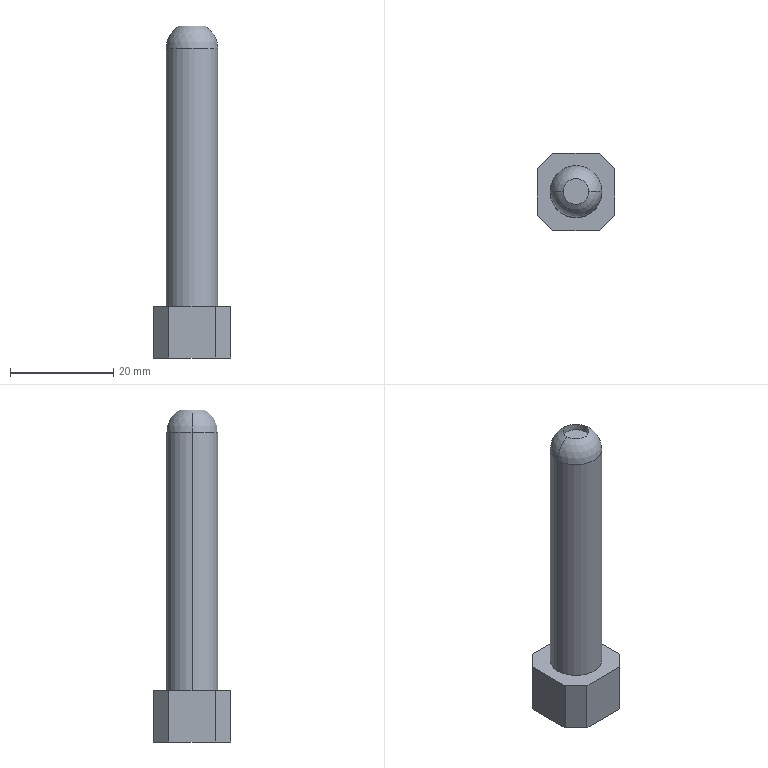Part | STEP file | Chamfer 1-56 | 1 solid | 17 faces | box 15 x 15 x 64.33 mm | volume 6226 mm3 | plane 11 | cylinder 4 | sphere 2 | commonest cylinder face diameters 5 x2 10 x2
STEP:
#1=CARTESIAN_POINT('',(-1533.738,1565.764,2844.751));
#2=VERTEX_POINT('',#1);
#3=CARTESIAN_POINT('',(-1528.738,1565.764,2844.751));
#4=VERTEX_POINT('',#3);
#5=CARTESIAN_POINT('',(-1531.238,1565.764,2844.751));
#6=DIRECTION('',(0.,0.,1.));
#7=DIRECTION('',(1.,0.,0.));
#8=AXIS2_PLACEMENT_3D('',#5,#6,#7);
#9=CIRCLE('',#8,2.5);
#10=EDGE_CURVE('',#2,#4,#9,.T.);
#11=ORIENTED_EDGE('',*,*,#10,.F.);
#12=CARTESIAN_POINT('',(-1533.738,1565.764,2846.081));
#13=VERTEX_POINT('',#12);
#14=CARTESIAN_POINT('',(-1533.738,1565.764,2844.751));
#15=DIRECTION('',(0.,0.,-1.));
#16=VECTOR('',#15,1000.);
#17=LINE('',#14,#16);
#18=EDGE_CURVE('',#13,#2,#17,.T.);
#19=ORIENTED_EDGE('',*,*,#18,.F.);
#20=CARTESIAN_POINT('',(-1528.738,1565.764,2846.081));
#21=VERTEX_POINT('',#20);
#22=CARTESIAN_POINT('',(-1531.238,1565.764,2846.081));
#23=DIRECTION('',(0.,0.,-1.));
#24=DIRECTION('',(-1.,0.,0.));
#25=AXIS2_PLACEMENT_3D('',#22,#23,#24);
#26=CIRCLE('',#25,2.5);
#27=EDGE_CURVE('',#21,#13,#26,.T.);
#28=ORIENTED_EDGE('',*,*,#27,.F.);
#29=CARTESIAN_POINT('',(-1528.738,1565.764,2844.751));
#30=DIRECTION('',(0.,0.,-1.));
#31=VECTOR('',#30,1000.);
#32=LINE('',#29,#31);
#33=EDGE_CURVE('',#21,#4,#32,.T.);
#34=ORIENTED_EDGE('',*,*,#33,.T.);
#35=EDGE_LOOP('',(#11,#19,#28,#34));
#36=FACE_OUTER_BOUND('',#35,.T.);
#37=CARTESIAN_POINT('',(-1531.238,1565.764,2844.751));
#38=DIRECTION('',(0.,0.,1.));
#39=DIRECTION('',(-1.,0.,0.));
#40=AXIS2_PLACEMENT_3D('',#37,#38,#39);
#41=CYLINDRICAL_SURFACE('',#40,2.5);
#42=ADVANCED_FACE('',(#36),#41,.F.);
#43=ORIENTED_EDGE('',*,*,#27,.T.);
#44=CARTESIAN_POINT('',(-1536.238,1565.764,2841.751));
#45=VERTEX_POINT('',#44);
#46=CARTESIAN_POINT('',(-1531.238,1565.764,2841.751));
#47=DIRECTION('',(0.,1.,0.));
#48=DIRECTION('',(1.,0.,0.));
#49=AXIS2_PLACEMENT_3D('',#46,#47,#48);
#50=CIRCLE('',#49,5.);
#51=EDGE_CURVE('',#45,#13,#50,.T.);
#52=ORIENTED_EDGE('',*,*,#51,.F.);
#53=CARTESIAN_POINT('',(-1526.238,1565.764,2841.751));
#54=VERTEX_POINT('',#53);
#55=CARTESIAN_POINT('',(-1531.238,1565.764,2841.751));
#56=DIRECTION('',(0.,0.,1.));
#57=DIRECTION('',(1.,0.,0.));
#58=AXIS2_PLACEMENT_3D('',#55,#56,#57);
#59=CIRCLE('',#58,5.);
#60=EDGE_CURVE('',#45,#54,#59,.T.);
#61=ORIENTED_EDGE('',*,*,#60,.T.);
#62=CARTESIAN_POINT('',(-1531.238,1565.764,2841.751));
#63=DIRECTION('',(0.,-1.,0.));
#64=DIRECTION('',(-1.,0.,0.));
#65=AXIS2_PLACEMENT_3D('',#62,#63,#64);
#66=CIRCLE('',#65,5.);
#67=EDGE_CURVE('',#54,#21,#66,.T.);
#68=ORIENTED_EDGE('',*,*,#67,.T.);
#69=EDGE_LOOP('',(#43,#52,#61,#68));
#70=FACE_OUTER_BOUND('',#69,.T.);
#71=CARTESIAN_POINT('',(-1531.238,1565.764,2841.751));
#72=DIRECTION('',(0.,0.,-1.));
#73=DIRECTION('',(-1.,0.,0.));
#74=AXIS2_PLACEMENT_3D('',#71,#72,#73);
#75=SPHERICAL_SURFACE('',#74,5.);
#76=ADVANCED_FACE('',(#70),#75,.T.);
#77=CARTESIAN_POINT('',(-1531.238,1565.764,2841.751));
#78=DIRECTION('',(0.,0.,1.));
#79=DIRECTION('',(1.,0.,0.));
#80=AXIS2_PLACEMENT_3D('',#77,#78,#79);
#81=CIRCLE('',#80,5.);
#82=EDGE_CURVE('',#54,#45,#81,.T.);
#83=ORIENTED_EDGE('',*,*,#82,.F.);
#84=CARTESIAN_POINT('',(-1526.238,1565.764,2791.751));
#85=VERTEX_POINT('',#84);
#86=CARTESIAN_POINT('',(-1526.238,1565.764,2841.751));
#87=DIRECTION('',(0.,0.,-1.));
#88=VECTOR('',#87,1000.);
#89=LINE('',#86,#88);
#90=EDGE_CURVE('',#54,#85,#89,.T.);
#91=ORIENTED_EDGE('',*,*,#90,.T.);
#92=CARTESIAN_POINT('',(-1536.238,1565.764,2791.751));
#93=VERTEX_POINT('',#92);
#94=CARTESIAN_POINT('',(-1531.238,1565.764,2791.751));
#95=DIRECTION('',(0.,0.,1.));
#96=DIRECTION('',(1.,0.,0.));
#97=AXIS2_PLACEMENT_3D('',#94,#95,#96);
#98=CIRCLE('',#97,5.);
#99=EDGE_CURVE('',#85,#93,#98,.T.);
#100=ORIENTED_EDGE('',*,*,#99,.T.);
#101=CARTESIAN_POINT('',(-1536.238,1565.764,2841.751));
#102=DIRECTION('',(0.,0.,-1.));
#103=VECTOR('',#102,1000.);
#104=LINE('',#101,#103);
#105=EDGE_CURVE('',#45,#93,#104,.T.);
#106=ORIENTED_EDGE('',*,*,#105,.F.);
#107=EDGE_LOOP('',(#83,#91,#100,#106));
#108=FACE_OUTER_BOUND('',#107,.T.);
#109=CARTESIAN_POINT('',(-1531.238,1565.764,2841.751));
#110=DIRECTION('',(0.,0.,-1.));
#111=DIRECTION('',(1.,0.,0.));
#112=AXIS2_PLACEMENT_3D('',#109,#110,#111);
#113=CYLINDRICAL_SURFACE('',#112,5.);
#114=ADVANCED_FACE('',(#108),#113,.T.);
#115=CARTESIAN_POINT('',(-1535.738,1558.264,2791.751));
#116=VERTEX_POINT('',#115);
#117=CARTESIAN_POINT('',(-1526.738,1558.264,2791.751));
#118=VERTEX_POINT('',#117);
#119=CARTESIAN_POINT('',(-1538.738,1558.264,2791.751));
#120=DIRECTION('',(1.,0.,0.));
#121=VECTOR('',#120,1000.);
#122=LINE('',#119,#121);
#123=EDGE_CURVE('',#116,#118,#122,.T.);
#124=ORIENTED_EDGE('',*,*,#123,.T.);
#125=CARTESIAN_POINT('',(-1523.738,1561.264,2791.751));
#126=VERTEX_POINT('',#125);
#127=CARTESIAN_POINT('',(-1525.238,1559.764,2791.751));
#128=DIRECTION('',(0.7071,0.7071,0.));
#129=VECTOR('',#128,1000.);
#130=LINE('',#127,#129);
#131=EDGE_CURVE('',#118,#126,#130,.T.);
#132=ORIENTED_EDGE('',*,*,#131,.T.);
#133=CARTESIAN_POINT('',(-1523.738,1570.264,2791.751));
#134=VERTEX_POINT('',#133);
#135=CARTESIAN_POINT('',(-1523.738,1573.264,2791.751));
#136=DIRECTION('',(0.,1.,0.));
#137=VECTOR('',#136,1000.);
#138=LINE('',#135,#137);
#139=EDGE_CURVE('',#126,#134,#138,.T.);
#140=ORIENTED_EDGE('',*,*,#139,.T.);
#141=CARTESIAN_POINT('',(-1526.738,1573.264,2791.751));
#142=VERTEX_POINT('',#141);
#143=CARTESIAN_POINT('',(-1525.238,1571.764,2791.751));
#144=DIRECTION('',(-0.7071,0.7071,0.));
#145=VECTOR('',#144,1000.);
#146=LINE('',#143,#145);
#147=EDGE_CURVE('',#134,#142,#146,.T.);
#148=ORIENTED_EDGE('',*,*,#147,.T.);
#149=CARTESIAN_POINT('',(-1535.738,1573.264,2791.751));
#150=VERTEX_POINT('',#149);
#151=CARTESIAN_POINT('',(-1538.738,1573.264,2791.751));
#152=DIRECTION('',(-1.,0.,0.));
#153=VECTOR('',#152,1000.);
#154=LINE('',#151,#153);
#155=EDGE_CURVE('',#142,#150,#154,.T.);
#156=ORIENTED_EDGE('',*,*,#155,.T.);
#157=CARTESIAN_POINT('',(-1538.738,1570.264,2791.751));
#158=VERTEX_POINT('',#157);
#159=CARTESIAN_POINT('',(-1537.238,1571.764,2791.751));
#160=DIRECTION('',(-0.7071,-0.7071,0.));
#161=VECTOR('',#160,1000.);
#162=LINE('',#159,#161);
#163=EDGE_CURVE('',#150,#158,#162,.T.);
#164=ORIENTED_EDGE('',*,*,#163,.T.);
#165=CARTESIAN_POINT('',(-1538.738,1561.264,2791.751));
#166=VERTEX_POINT('',#165);
#167=CARTESIAN_POINT('',(-1538.738,1573.264,2791.751));
#168=DIRECTION('',(0.,-1.,0.));
#169=VECTOR('',#168,1000.);
#170=LINE('',#167,#169);
#171=EDGE_CURVE('',#158,#166,#170,.T.);
#172=ORIENTED_EDGE('',*,*,#171,.T.);
#173=CARTESIAN_POINT('',(-1537.238,1559.764,2791.751));
#174=DIRECTION('',(0.7071,-0.7071,0.));
#175=VECTOR('',#174,1000.);
#176=LINE('',#173,#175);
#177=EDGE_CURVE('',#166,#116,#176,.T.);
#178=ORIENTED_EDGE('',*,*,#177,.T.);
#179=EDGE_LOOP('',(#124,#132,#140,#148,#156,#164,#172,#178));
#180=FACE_OUTER_BOUND('',#179,.T.);
#181=CARTESIAN_POINT('',(-1531.238,1565.764,2791.751));
#182=DIRECTION('',(0.,0.,1.));
#183=DIRECTION('',(1.,0.,0.));
#184=AXIS2_PLACEMENT_3D('',#181,#182,#183);
#185=CIRCLE('',#184,5.);
#186=EDGE_CURVE('',#93,#85,#185,.T.);
#187=ORIENTED_EDGE('',*,*,#186,.F.);
#188=ORIENTED_EDGE('',*,*,#99,.F.);
#189=EDGE_LOOP('',(#187,#188));
#190=FACE_BOUND('',#189,.T.);
#191=CARTESIAN_POINT('',(-1531.238,1565.764,2791.751));
#192=DIRECTION('',(0.,0.,1.));
#193=DIRECTION('',(-1.,0.,0.));
#194=AXIS2_PLACEMENT_3D('',#191,#192,#193);
#195=PLANE('',#194);
#196=ADVANCED_FACE('',(#180,#190),#195,.T.);
#197=ORIENTED_EDGE('',*,*,#139,.F.);
#198=CARTESIAN_POINT('',(-1523.738,1561.264,2781.751));
#199=VERTEX_POINT('',#198);
#200=CARTESIAN_POINT('',(-1523.738,1561.264,2791.751));
#201=DIRECTION('',(0.,0.,-1.));
#202=VECTOR('',#201,1000.);
#203=LINE('',#200,#202);
#204=EDGE_CURVE('',#126,#199,#203,.T.);
#205=ORIENTED_EDGE('',*,*,#204,.T.);
#206=CARTESIAN_POINT('',(-1523.738,1570.264,2781.751));
#207=VERTEX_POINT('',#206);
#208=CARTESIAN_POINT('',(-1523.738,1573.264,2781.751));
#209=DIRECTION('',(0.,1.,0.));
#210=VECTOR('',#209,1000.);
#211=LINE('',#208,#210);
#212=EDGE_CURVE('',#199,#207,#211,.T.);
#213=ORIENTED_EDGE('',*,*,#212,.T.);
#214=CARTESIAN_POINT('',(-1523.738,1570.264,2791.751));
#215=DIRECTION('',(0.,0.,1.));
#216=VECTOR('',#215,1000.);
#217=LINE('',#214,#216);
#218=EDGE_CURVE('',#207,#134,#217,.T.);
#219=ORIENTED_EDGE('',*,*,#218,.T.);
#220=EDGE_LOOP('',(#197,#205,#213,#219));
#221=FACE_OUTER_BOUND('',#220,.T.);
#222=CARTESIAN_POINT('',(-1523.738,1573.264,2791.751));
#223=DIRECTION('',(-1.,0.,0.));
#224=DIRECTION('',(0.,1.,0.));
#225=AXIS2_PLACEMENT_3D('',#222,#223,#224);
#226=PLANE('',#225);
#227=ADVANCED_FACE('',(#221),#226,.F.);
#228=CARTESIAN_POINT('',(-1526.738,1573.264,2781.751));
#229=VERTEX_POINT('',#228);
#230=CARTESIAN_POINT('',(-1535.738,1573.264,2781.751));
#231=VERTEX_POINT('',#230);
#232=CARTESIAN_POINT('',(-1538.738,1573.264,2781.751));
#233=DIRECTION('',(-1.,0.,0.));
#234=VECTOR('',#233,1000.);
#235=LINE('',#232,#234);
#236=EDGE_CURVE('',#229,#231,#235,.T.);
#237=ORIENTED_EDGE('',*,*,#236,.T.);
#238=CARTESIAN_POINT('',(-1535.738,1573.264,2791.751));
#239=DIRECTION('',(0.,0.,1.));
#240=VECTOR('',#239,1000.);
#241=LINE('',#238,#240);
#242=EDGE_CURVE('',#231,#150,#241,.T.);
#243=ORIENTED_EDGE('',*,*,#242,.T.);
#244=ORIENTED_EDGE('',*,*,#155,.F.);
#245=CARTESIAN_POINT('',(-1526.738,1573.264,2791.751));
#246=DIRECTION('',(0.,0.,-1.));
#247=VECTOR('',#246,1000.);
#248=LINE('',#245,#247);
#249=EDGE_CURVE('',#142,#229,#248,.T.);
#250=ORIENTED_EDGE('',*,*,#249,.T.);
#251=EDGE_LOOP('',(#237,#243,#244,#250));
#252=FACE_OUTER_BOUND('',#251,.T.);
#253=CARTESIAN_POINT('',(-1538.738,1573.264,2791.751));
#254=DIRECTION('',(0.,-1.,0.));
#255=DIRECTION('',(-1.,0.,0.));
#256=AXIS2_PLACEMENT_3D('',#253,#254,#255);
#257=PLANE('',#256);
#258=ADVANCED_FACE('',(#252),#257,.F.);
#259=CARTESIAN_POINT('',(-1538.738,1570.264,2781.751));
#260=VERTEX_POINT('',#259);
#261=CARTESIAN_POINT('',(-1538.738,1561.264,2781.751));
#262=VERTEX_POINT('',#261);
#263=CARTESIAN_POINT('',(-1538.738,1573.264,2781.751));
#264=DIRECTION('',(0.,-1.,0.));
#265=VECTOR('',#264,1000.);
#266=LINE('',#263,#265);
#267=EDGE_CURVE('',#260,#262,#266,.T.);
#268=ORIENTED_EDGE('',*,*,#267,.T.);
#269=CARTESIAN_POINT('',(-1538.738,1561.264,2791.751));
#270=DIRECTION('',(0.,0.,1.));
#271=VECTOR('',#270,1000.);
#272=LINE('',#269,#271);
#273=EDGE_CURVE('',#262,#166,#272,.T.);
#274=ORIENTED_EDGE('',*,*,#273,.T.);
#275=ORIENTED_EDGE('',*,*,#171,.F.);
#276=CARTESIAN_POINT('',(-1538.738,1570.264,2791.751));
#277=DIRECTION('',(0.,0.,-1.));
#278=VECTOR('',#277,1000.);
#279=LINE('',#276,#278);
#280=EDGE_CURVE('',#158,#260,#279,.T.);
#281=ORIENTED_EDGE('',*,*,#280,.T.);
#282=EDGE_LOOP('',(#268,#274,#275,#281));
#283=FACE_OUTER_BOUND('',#282,.T.);
#284=CARTESIAN_POINT('',(-1538.738,1573.264,2791.751));
#285=DIRECTION('',(1.,0.,0.));
#286=DIRECTION('',(0.,-1.,0.));
#287=AXIS2_PLACEMENT_3D('',#284,#285,#286);
#288=PLANE('',#287);
#289=ADVANCED_FACE('',(#283),#288,.F.);
#290=CARTESIAN_POINT('',(-1535.738,1558.264,2781.751));
#291=VERTEX_POINT('',#290);
#292=CARTESIAN_POINT('',(-1526.738,1558.264,2781.751));
#293=VERTEX_POINT('',#292);
#294=CARTESIAN_POINT('',(-1538.738,1558.264,2781.751));
#295=DIRECTION('',(1.,0.,0.));
#296=VECTOR('',#295,1000.);
#297=LINE('',#294,#296);
#298=EDGE_CURVE('',#291,#293,#297,.T.);
#299=ORIENTED_EDGE('',*,*,#298,.T.);
#300=CARTESIAN_POINT('',(-1526.738,1558.264,2791.751));
#301=DIRECTION('',(0.,0.,1.));
#302=VECTOR('',#301,1000.);
#303=LINE('',#300,#302);
#304=EDGE_CURVE('',#293,#118,#303,.T.);
#305=ORIENTED_EDGE('',*,*,#304,.T.);
#306=ORIENTED_EDGE('',*,*,#123,.F.);
#307=CARTESIAN_POINT('',(-1535.738,1558.264,2791.751));
#308=DIRECTION('',(0.,0.,-1.));
#309=VECTOR('',#308,1000.);
#310=LINE('',#307,#309);
#311=EDGE_CURVE('',#116,#291,#310,.T.);
#312=ORIENTED_EDGE('',*,*,#311,.T.);
#313=EDGE_LOOP('',(#299,#305,#306,#312));
#314=FACE_OUTER_BOUND('',#313,.T.);
#315=CARTESIAN_POINT('',(-1538.738,1558.264,2791.751));
#316=DIRECTION('',(0.,1.,0.));
#317=DIRECTION('',(1.,0.,0.));
#318=AXIS2_PLACEMENT_3D('',#315,#316,#317);
#319=PLANE('',#318);
#320=ADVANCED_FACE('',(#314),#319,.F.);
#321=ORIENTED_EDGE('',*,*,#212,.F.);
#322=CARTESIAN_POINT('',(-1523.738,1561.264,2781.751));
#323=DIRECTION('',(-0.7071,-0.7071,0.));
#324=VECTOR('',#323,1000.);
#325=LINE('',#322,#324);
#326=EDGE_CURVE('',#199,#293,#325,.T.);
#327=ORIENTED_EDGE('',*,*,#326,.T.);
#328=ORIENTED_EDGE('',*,*,#298,.F.);
#329=CARTESIAN_POINT('',(-1535.738,1558.264,2781.751));
#330=DIRECTION('',(-0.7071,0.7071,0.));
#331=VECTOR('',#330,1000.);
#332=LINE('',#329,#331);
#333=EDGE_CURVE('',#291,#262,#332,.T.);
#334=ORIENTED_EDGE('',*,*,#333,.T.);
#335=ORIENTED_EDGE('',*,*,#267,.F.);
#336=CARTESIAN_POINT('',(-1538.738,1570.264,2781.751));
#337=DIRECTION('',(0.7071,0.7071,0.));
#338=VECTOR('',#337,1000.);
#339=LINE('',#336,#338);
#340=EDGE_CURVE('',#260,#231,#339,.T.);
#341=ORIENTED_EDGE('',*,*,#340,.T.);
#342=ORIENTED_EDGE('',*,*,#236,.F.);
#343=CARTESIAN_POINT('',(-1526.738,1573.264,2781.751));
#344=DIRECTION('',(0.7071,-0.7071,0.));
#345=VECTOR('',#344,1000.);
#346=LINE('',#343,#345);
#347=EDGE_CURVE('',#229,#207,#346,.T.);
#348=ORIENTED_EDGE('',*,*,#347,.T.);
#349=EDGE_LOOP('',(#321,#327,#328,#334,#335,#341,#342,#348));
#350=FACE_OUTER_BOUND('',#349,.T.);
#351=CARTESIAN_POINT('',(-1531.238,1565.764,2781.751));
#352=DIRECTION('',(0.,0.,1.));
#353=DIRECTION('',(-1.,0.,0.));
#354=AXIS2_PLACEMENT_3D('',#351,#352,#353);
#355=PLANE('',#354);
#356=ADVANCED_FACE('',(#350),#355,.F.);
#357=ORIENTED_EDGE('',*,*,#90,.F.);
#358=ORIENTED_EDGE('',*,*,#60,.F.);
#359=ORIENTED_EDGE('',*,*,#105,.T.);
#360=ORIENTED_EDGE('',*,*,#186,.T.);
#361=EDGE_LOOP('',(#357,#358,#359,#360));
#362=FACE_OUTER_BOUND('',#361,.T.);
#363=CARTESIAN_POINT('',(-1531.238,1565.764,2841.751));
#364=DIRECTION('',(0.,0.,-1.));
#365=DIRECTION('',(1.,0.,0.));
#366=AXIS2_PLACEMENT_3D('',#363,#364,#365);
#367=CYLINDRICAL_SURFACE('',#366,5.);
#368=ADVANCED_FACE('',(#362),#367,.T.);
#369=ORIENTED_EDGE('',*,*,#51,.T.);
#370=CARTESIAN_POINT('',(-1531.238,1565.764,2846.081));
#371=DIRECTION('',(0.,0.,-1.));
#372=DIRECTION('',(-1.,0.,0.));
#373=AXIS2_PLACEMENT_3D('',#370,#371,#372);
#374=CIRCLE('',#373,2.5);
#375=EDGE_CURVE('',#13,#21,#374,.T.);
#376=ORIENTED_EDGE('',*,*,#375,.T.);
#377=ORIENTED_EDGE('',*,*,#67,.F.);
#378=ORIENTED_EDGE('',*,*,#82,.T.);
#379=EDGE_LOOP('',(#369,#376,#377,#378));
#380=FACE_OUTER_BOUND('',#379,.T.);
#381=CARTESIAN_POINT('',(-1531.238,1565.764,2841.751));
#382=DIRECTION('',(0.,0.,-1.));
#383=DIRECTION('',(-1.,0.,0.));
#384=AXIS2_PLACEMENT_3D('',#381,#382,#383);
#385=SPHERICAL_SURFACE('',#384,5.);
#386=ADVANCED_FACE('',(#380),#385,.T.);
#387=ORIENTED_EDGE('',*,*,#18,.T.);
#388=CARTESIAN_POINT('',(-1531.238,1565.764,2844.751));
#389=DIRECTION('',(0.,0.,1.));
#390=DIRECTION('',(1.,0.,0.));
#391=AXIS2_PLACEMENT_3D('',#388,#389,#390);
#392=CIRCLE('',#391,2.5);
#393=EDGE_CURVE('',#4,#2,#392,.T.);
#394=ORIENTED_EDGE('',*,*,#393,.F.);
#395=ORIENTED_EDGE('',*,*,#33,.F.);
#396=ORIENTED_EDGE('',*,*,#375,.F.);
#397=EDGE_LOOP('',(#387,#394,#395,#396));
#398=FACE_OUTER_BOUND('',#397,.T.);
#399=CARTESIAN_POINT('',(-1531.238,1565.764,2844.751));
#400=DIRECTION('',(0.,0.,1.));
#401=DIRECTION('',(-1.,0.,0.));
#402=AXIS2_PLACEMENT_3D('',#399,#400,#401);
#403=CYLINDRICAL_SURFACE('',#402,2.5);
#404=ADVANCED_FACE('',(#398),#403,.F.);
#405=ORIENTED_EDGE('',*,*,#393,.T.);
#406=ORIENTED_EDGE('',*,*,#10,.T.);
#407=EDGE_LOOP('',(#405,#406));
#408=FACE_OUTER_BOUND('',#407,.T.);
#409=CARTESIAN_POINT('',(-1531.238,1565.764,2844.751));
#410=DIRECTION('',(0.,0.,1.));
#411=DIRECTION('',(-1.,0.,0.));
#412=AXIS2_PLACEMENT_3D('',#409,#410,#411);
#413=PLANE('',#412);
#414=ADVANCED_FACE('',(#408),#413,.T.);
#415=ORIENTED_EDGE('',*,*,#131,.F.);
#416=ORIENTED_EDGE('',*,*,#304,.F.);
#417=ORIENTED_EDGE('',*,*,#326,.F.);
#418=ORIENTED_EDGE('',*,*,#204,.F.);
#419=EDGE_LOOP('',(#415,#416,#417,#418));
#420=FACE_OUTER_BOUND('',#419,.T.);
#421=CARTESIAN_POINT('',(-1523.738,1561.264,2791.751));
#422=DIRECTION('',(-0.7071,0.7071,0.));
#423=DIRECTION('',(0.,0.,1.));
#424=AXIS2_PLACEMENT_3D('',#421,#422,#423);
#425=PLANE('',#424);
#426=ADVANCED_FACE('',(#420),#425,.F.);
#427=ORIENTED_EDGE('',*,*,#177,.F.);
#428=ORIENTED_EDGE('',*,*,#273,.F.);
#429=ORIENTED_EDGE('',*,*,#333,.F.);
#430=ORIENTED_EDGE('',*,*,#311,.F.);
#431=EDGE_LOOP('',(#427,#428,#429,#430));
#432=FACE_OUTER_BOUND('',#431,.T.);
#433=CARTESIAN_POINT('',(-1535.738,1558.264,2791.751));
#434=DIRECTION('',(0.7071,0.7071,0.));
#435=DIRECTION('',(0.,0.,1.));
#436=AXIS2_PLACEMENT_3D('',#433,#434,#435);
#437=PLANE('',#436);
#438=ADVANCED_FACE('',(#432),#437,.F.);
#439=ORIENTED_EDGE('',*,*,#163,.F.);
#440=ORIENTED_EDGE('',*,*,#242,.F.);
#441=ORIENTED_EDGE('',*,*,#340,.F.);
#442=ORIENTED_EDGE('',*,*,#280,.F.);
#443=EDGE_LOOP('',(#439,#440,#441,#442));
#444=FACE_OUTER_BOUND('',#443,.T.);
#445=CARTESIAN_POINT('',(-1538.738,1570.264,2791.751));
#446=DIRECTION('',(0.7071,-0.7071,0.));
#447=DIRECTION('',(0.,0.,1.));
#448=AXIS2_PLACEMENT_3D('',#445,#446,#447);
#449=PLANE('',#448);
#450=ADVANCED_FACE('',(#444),#449,.F.);
#451=ORIENTED_EDGE('',*,*,#147,.F.);
#452=ORIENTED_EDGE('',*,*,#218,.F.);
#453=ORIENTED_EDGE('',*,*,#347,.F.);
#454=ORIENTED_EDGE('',*,*,#249,.F.);
#455=EDGE_LOOP('',(#451,#452,#453,#454));
#456=FACE_OUTER_BOUND('',#455,.T.);
#457=CARTESIAN_POINT('',(-1526.738,1573.264,2791.751));
#458=DIRECTION('',(-0.7071,-0.7071,0.));
#459=DIRECTION('',(0.,0.,1.));
#460=AXIS2_PLACEMENT_3D('',#457,#458,#459);
#461=PLANE('',#460);
#462=ADVANCED_FACE('',(#456),#461,.F.);
#463=CLOSED_SHELL('',(#42,#76,#114,#196,#227,#258,#289,#320,#356,#368,#386,#404,#414,#426,#438,#450,#462));
#464=MANIFOLD_SOLID_BREP('',#463);
#465=CARTESIAN_POINT('',(0.,0.,0.));
#466=DIRECTION('',(0.,0.,1.));
#467=DIRECTION('',(1.,0.,0.));
#468=AXIS2_PLACEMENT_3D('',#465,#466,#467);
#469=(LENGTH_UNIT()NAMED_UNIT(*)SI_UNIT(.MILLI.,.METRE.));
#470=UNCERTAINTY_MEASURE_WITH_UNIT(LENGTH_MEASURE(0.00001),#469,'','');
#471=(NAMED_UNIT(*)PLANE_ANGLE_UNIT()SI_UNIT($,.RADIAN.));
#472=(NAMED_UNIT(*)SI_UNIT($,.STERADIAN.)SOLID_ANGLE_UNIT());
#473=(GEOMETRIC_REPRESENTATION_CONTEXT(3)GLOBAL_UNCERTAINTY_ASSIGNED_CONTEXT((#470))GLOBAL_UNIT_ASSIGNED_CONTEXT((#469,#471,#472))REPRESENTATION_CONTEXT('',''));
#474=ADVANCED_BREP_SHAPE_REPRESENTATION('',(#464,#468),#473);